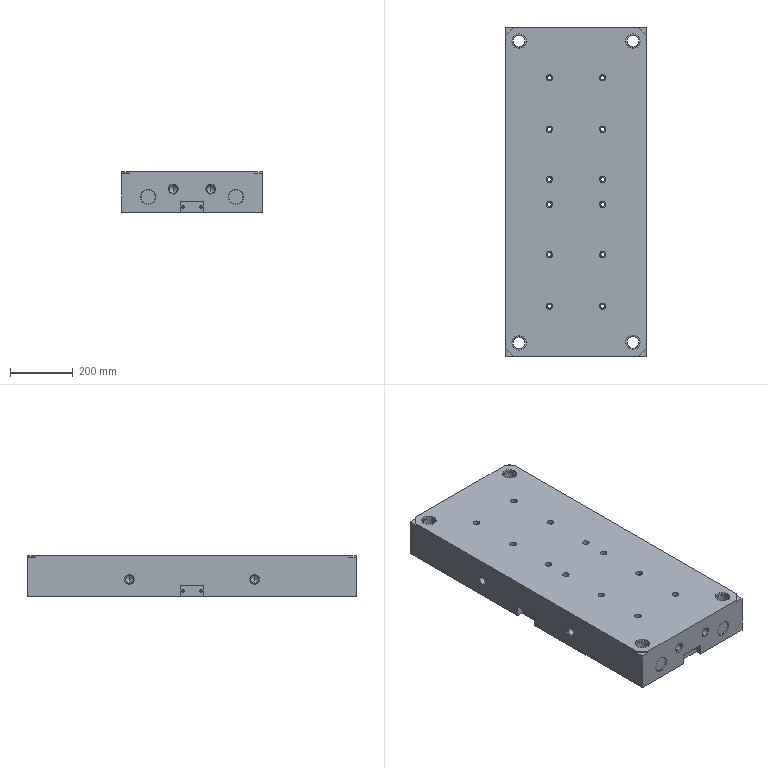Part | STEP file | 4-20.sldasm-Part-423 | 1 solid | 273 faces | box 450 x 1050 x 130 mm | volume 42151438 mm3 | cylinder 126 | plane 73 | cone 70 | torus 4 | commonest cylinder face diameters 13.492 x24 20.638 x24 8.237 x16 25.4 x16 8 x8 15 x8